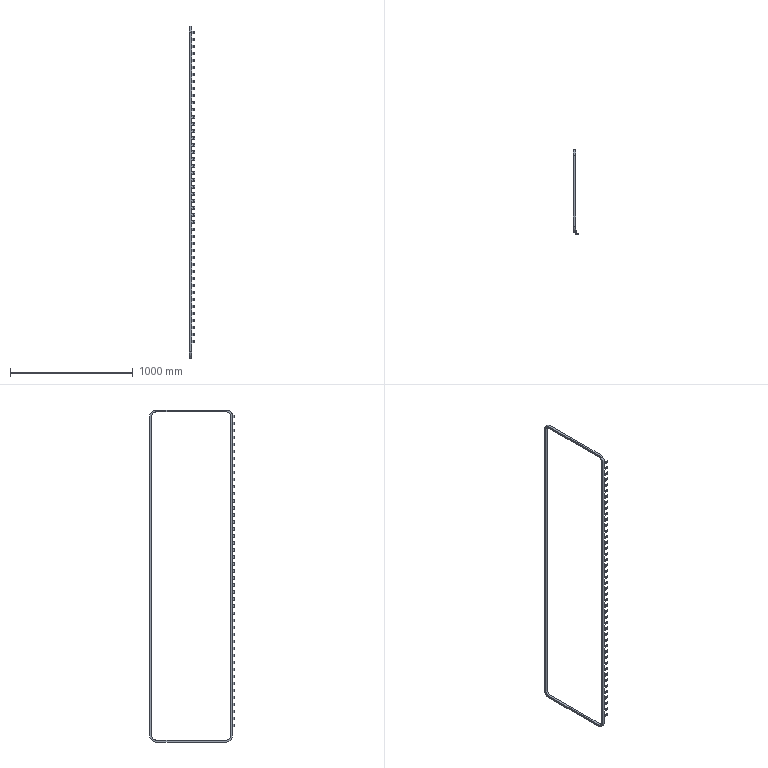Part | SolidWorks | features ICE 2, ExtruThin 1, HoleWzd 1, LPattern 1 | 1 solid | 467 faces | box 41.8 x 686 x 2700 mm | volume 2120654 mm3 | plane 369 | cylinder 98 | commonest cylinder face diameters 4.2 x90 67.62 x4 99.62 x4